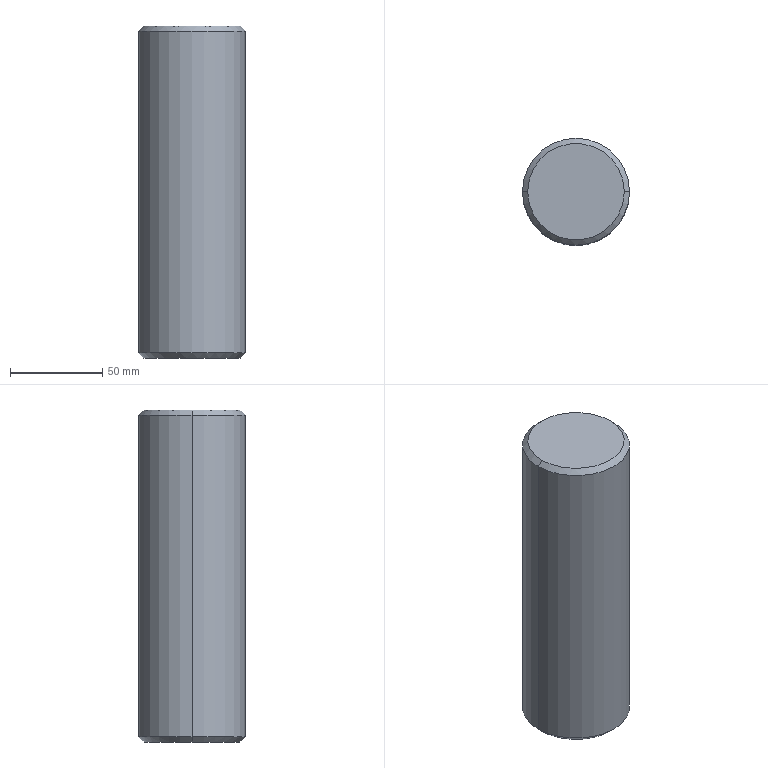Part | SolidWorks | features BaseBody 1 | 1 solid | 12 faces | box 58 x 58 x 180 mm | volume 471042 mm3 | cone 6 | cylinder 4 | plane 2 | commonest cylinder face diameters 10.5 x2 58 x2
STEP:
#1=CARTESIAN_POINT('',(74.754,163.004,-390.5));
#2=VERTEX_POINT('',#1);
#3=CARTESIAN_POINT('',(85.254,163.004,-390.5));
#4=VERTEX_POINT('',#3);
#5=CARTESIAN_POINT('',(80.004,163.004,-390.5));
#6=DIRECTION('',(0.,0.,1.));
#7=DIRECTION('',(1.,0.,0.));
#8=AXIS2_PLACEMENT_3D('',#5,#6,#7);
#9=CIRCLE('',#8,5.25);
#10=EDGE_CURVE('',#2,#4,#9,.T.);
#11=ORIENTED_EDGE('',*,*,#10,.F.);
#12=CARTESIAN_POINT('',(74.754,163.004,-355.5));
#13=VERTEX_POINT('',#12);
#14=CARTESIAN_POINT('',(74.754,163.004,-390.5));
#15=DIRECTION('',(0.,0.,1.));
#16=VECTOR('',#15,1000.);
#17=LINE('',#14,#16);
#18=EDGE_CURVE('',#2,#13,#17,.T.);
#19=ORIENTED_EDGE('',*,*,#18,.T.);
#20=CARTESIAN_POINT('',(85.254,163.004,-355.5));
#21=VERTEX_POINT('',#20);
#22=CARTESIAN_POINT('',(80.004,163.004,-355.5));
#23=DIRECTION('',(0.,0.,1.));
#24=DIRECTION('',(1.,0.,0.));
#25=AXIS2_PLACEMENT_3D('',#22,#23,#24);
#26=CIRCLE('',#25,5.25);
#27=EDGE_CURVE('',#13,#21,#26,.T.);
#28=ORIENTED_EDGE('',*,*,#27,.T.);
#29=CARTESIAN_POINT('',(85.254,163.004,-390.5));
#30=DIRECTION('',(0.,0.,1.));
#31=VECTOR('',#30,1000.);
#32=LINE('',#29,#31);
#33=EDGE_CURVE('',#4,#21,#32,.T.);
#34=ORIENTED_EDGE('',*,*,#33,.F.);
#35=EDGE_LOOP('',(#11,#19,#28,#34));
#36=FACE_OUTER_BOUND('',#35,.T.);
#37=CARTESIAN_POINT('',(80.004,163.004,-390.5));
#38=DIRECTION('',(0.,0.,1.));
#39=DIRECTION('',(1.,0.,0.));
#40=AXIS2_PLACEMENT_3D('',#37,#38,#39);
#41=CYLINDRICAL_SURFACE('',#40,5.25);
#42=ADVANCED_FACE('',(#36),#41,.F.);
#43=CARTESIAN_POINT('',(80.004,163.004,-352.345));
#44=VERTEX_POINT('',#43);
#45=CARTESIAN_POINT('',(74.754,163.004,-355.5));
#46=DIRECTION('',(-0.8572,0.,-0.515));
#47=VECTOR('',#46,1000.);
#48=LINE('',#45,#47);
#49=EDGE_CURVE('',#44,#13,#48,.T.);
#50=ORIENTED_EDGE('',*,*,#49,.F.);
#51=CARTESIAN_POINT('',(85.254,163.004,-355.5));
#52=DIRECTION('',(0.8572,0.,-0.515));
#53=VECTOR('',#52,1000.);
#54=LINE('',#51,#53);
#55=EDGE_CURVE('',#44,#21,#54,.T.);
#56=ORIENTED_EDGE('',*,*,#55,.T.);
#57=ORIENTED_EDGE('',*,*,#27,.F.);
#58=EDGE_LOOP('',(#50,#56,#57));
#59=FACE_OUTER_BOUND('',#58,.T.);
#60=CARTESIAN_POINT('',(80.004,163.004,-355.5));
#61=DIRECTION('',(0.,0.,-1.));
#62=DIRECTION('',(-1.,0.,0.));
#63=AXIS2_PLACEMENT_3D('',#60,#61,#62);
#64=CONICAL_SURFACE('',#63,5.25,1.03);
#65=ADVANCED_FACE('',(#59),#64,.F.);
#66=CARTESIAN_POINT('',(53.832,163.004,-390.5));
#67=VERTEX_POINT('',#66);
#68=CARTESIAN_POINT('',(106.175,163.004,-390.5));
#69=VERTEX_POINT('',#68);
#70=CARTESIAN_POINT('',(80.004,163.004,-390.5));
#71=DIRECTION('',(0.,0.,-1.));
#72=DIRECTION('',(1.,0.,0.));
#73=AXIS2_PLACEMENT_3D('',#70,#71,#72);
#74=CIRCLE('',#73,26.172);
#75=EDGE_CURVE('',#67,#69,#74,.T.);
#76=ORIENTED_EDGE('',*,*,#75,.F.);
#77=CARTESIAN_POINT('',(51.004,163.004,-387.672));
#78=VERTEX_POINT('',#77);
#79=CARTESIAN_POINT('',(50.418,163.004,-387.086));
#80=DIRECTION('',(-0.7071,0.,0.7071));
#81=VECTOR('',#80,1000.);
#82=LINE('',#79,#81);
#83=EDGE_CURVE('',#67,#78,#82,.T.);
#84=ORIENTED_EDGE('',*,*,#83,.T.);
#85=CARTESIAN_POINT('',(109.004,163.004,-387.672));
#86=VERTEX_POINT('',#85);
#87=CARTESIAN_POINT('',(80.004,163.004,-387.672));
#88=DIRECTION('',(0.,0.,1.));
#89=DIRECTION('',(1.,0.,0.));
#90=AXIS2_PLACEMENT_3D('',#87,#88,#89);
#91=CIRCLE('',#90,29.);
#92=EDGE_CURVE('',#86,#78,#91,.T.);
#93=ORIENTED_EDGE('',*,*,#92,.F.);
#94=CARTESIAN_POINT('',(109.589,163.004,-387.086));
#95=DIRECTION('',(0.7071,0.,0.7071));
#96=VECTOR('',#95,1000.);
#97=LINE('',#94,#96);
#98=EDGE_CURVE('',#69,#86,#97,.T.);
#99=ORIENTED_EDGE('',*,*,#98,.F.);
#100=EDGE_LOOP('',(#76,#84,#93,#99));
#101=FACE_OUTER_BOUND('',#100,.T.);
#102=CARTESIAN_POINT('',(80.004,163.004,-387.086));
#103=DIRECTION('',(0.,0.,1.));
#104=DIRECTION('',(1.,0.,0.));
#105=AXIS2_PLACEMENT_3D('',#102,#103,#104);
#106=CONICAL_SURFACE('',#105,29.586,0.7854);
#107=ADVANCED_FACE('',(#101),#106,.T.);
#108=CARTESIAN_POINT('',(106.175,163.004,-210.5));
#109=VERTEX_POINT('',#108);
#110=CARTESIAN_POINT('',(53.832,163.004,-210.5));
#111=VERTEX_POINT('',#110);
#112=CARTESIAN_POINT('',(80.004,163.004,-210.5));
#113=DIRECTION('',(0.,0.,1.));
#114=DIRECTION('',(1.,0.,0.));
#115=AXIS2_PLACEMENT_3D('',#112,#113,#114);
#116=CIRCLE('',#115,26.172);
#117=EDGE_CURVE('',#109,#111,#116,.T.);
#118=ORIENTED_EDGE('',*,*,#117,.F.);
#119=CARTESIAN_POINT('',(109.004,163.004,-213.328));
#120=VERTEX_POINT('',#119);
#121=CARTESIAN_POINT('',(107.589,163.004,-211.914));
#122=DIRECTION('',(0.7071,0.,-0.7071));
#123=VECTOR('',#122,1000.);
#124=LINE('',#121,#123);
#125=EDGE_CURVE('',#109,#120,#124,.T.);
#126=ORIENTED_EDGE('',*,*,#125,.T.);
#127=CARTESIAN_POINT('',(51.004,163.004,-213.328));
#128=VERTEX_POINT('',#127);
#129=CARTESIAN_POINT('',(80.004,163.004,-213.328));
#130=DIRECTION('',(0.,0.,-1.));
#131=DIRECTION('',(-1.,0.,0.));
#132=AXIS2_PLACEMENT_3D('',#129,#130,#131);
#133=CIRCLE('',#132,29.);
#134=EDGE_CURVE('',#128,#120,#133,.T.);
#135=ORIENTED_EDGE('',*,*,#134,.F.);
#136=CARTESIAN_POINT('',(52.418,163.004,-211.914));
#137=DIRECTION('',(-0.7071,0.,-0.7071));
#138=VECTOR('',#137,1000.);
#139=LINE('',#136,#138);
#140=EDGE_CURVE('',#111,#128,#139,.T.);
#141=ORIENTED_EDGE('',*,*,#140,.F.);
#142=EDGE_LOOP('',(#118,#126,#135,#141));
#143=FACE_OUTER_BOUND('',#142,.T.);
#144=CARTESIAN_POINT('',(80.004,163.004,-211.914));
#145=DIRECTION('',(0.,0.,-1.));
#146=DIRECTION('',(-1.,0.,0.));
#147=AXIS2_PLACEMENT_3D('',#144,#145,#146);
#148=CONICAL_SURFACE('',#147,27.586,0.7854);
#149=ADVANCED_FACE('',(#143),#148,.T.);
#150=ORIENTED_EDGE('',*,*,#134,.T.);
#151=CARTESIAN_POINT('',(109.004,163.004,-210.5));
#152=DIRECTION('',(0.,0.,-1.));
#153=VECTOR('',#152,1000.);
#154=LINE('',#151,#153);
#155=EDGE_CURVE('',#120,#86,#154,.T.);
#156=ORIENTED_EDGE('',*,*,#155,.T.);
#157=ORIENTED_EDGE('',*,*,#92,.T.);
#158=CARTESIAN_POINT('',(51.004,163.004,-210.5));
#159=DIRECTION('',(0.,0.,-1.));
#160=VECTOR('',#159,1000.);
#161=LINE('',#158,#160);
#162=EDGE_CURVE('',#128,#78,#161,.T.);
#163=ORIENTED_EDGE('',*,*,#162,.F.);
#164=EDGE_LOOP('',(#150,#156,#157,#163));
#165=FACE_OUTER_BOUND('',#164,.T.);
#166=CARTESIAN_POINT('',(80.004,163.004,-210.5));
#167=DIRECTION('',(0.,0.,-1.));
#168=DIRECTION('',(-1.,0.,0.));
#169=AXIS2_PLACEMENT_3D('',#166,#167,#168);
#170=CYLINDRICAL_SURFACE('',#169,29.);
#171=ADVANCED_FACE('',(#165),#170,.T.);
#172=ORIENTED_EDGE('',*,*,#155,.F.);
#173=CARTESIAN_POINT('',(80.004,163.004,-213.328));
#174=DIRECTION('',(0.,0.,-1.));
#175=DIRECTION('',(-1.,0.,0.));
#176=AXIS2_PLACEMENT_3D('',#173,#174,#175);
#177=CIRCLE('',#176,29.);
#178=EDGE_CURVE('',#120,#128,#177,.T.);
#179=ORIENTED_EDGE('',*,*,#178,.T.);
#180=ORIENTED_EDGE('',*,*,#162,.T.);
#181=CARTESIAN_POINT('',(80.004,163.004,-387.672));
#182=DIRECTION('',(0.,0.,1.));
#183=DIRECTION('',(1.,0.,0.));
#184=AXIS2_PLACEMENT_3D('',#181,#182,#183);
#185=CIRCLE('',#184,29.);
#186=EDGE_CURVE('',#78,#86,#185,.T.);
#187=ORIENTED_EDGE('',*,*,#186,.T.);
#188=EDGE_LOOP('',(#172,#179,#180,#187));
#189=FACE_OUTER_BOUND('',#188,.T.);
#190=CARTESIAN_POINT('',(80.004,163.004,-210.5));
#191=DIRECTION('',(0.,0.,-1.));
#192=DIRECTION('',(-1.,0.,0.));
#193=AXIS2_PLACEMENT_3D('',#190,#191,#192);
#194=CYLINDRICAL_SURFACE('',#193,29.);
#195=ADVANCED_FACE('',(#189),#194,.T.);
#196=CARTESIAN_POINT('',(80.004,163.004,-210.5));
#197=DIRECTION('',(0.,0.,1.));
#198=DIRECTION('',(1.,0.,0.));
#199=AXIS2_PLACEMENT_3D('',#196,#197,#198);
#200=CIRCLE('',#199,26.172);
#201=EDGE_CURVE('',#111,#109,#200,.T.);
#202=ORIENTED_EDGE('',*,*,#201,.T.);
#203=ORIENTED_EDGE('',*,*,#117,.T.);
#204=EDGE_LOOP('',(#202,#203));
#205=FACE_OUTER_BOUND('',#204,.T.);
#206=CARTESIAN_POINT('',(80.004,163.004,-210.5));
#207=DIRECTION('',(0.,0.,1.));
#208=DIRECTION('',(1.,0.,0.));
#209=AXIS2_PLACEMENT_3D('',#206,#207,#208);
#210=PLANE('',#209);
#211=ADVANCED_FACE('',(#205),#210,.T.);
#212=CARTESIAN_POINT('',(80.004,163.004,-390.5));
#213=DIRECTION('',(0.,0.,1.));
#214=DIRECTION('',(1.,0.,0.));
#215=AXIS2_PLACEMENT_3D('',#212,#213,#214);
#216=CIRCLE('',#215,5.25);
#217=EDGE_CURVE('',#4,#2,#216,.T.);
#218=ORIENTED_EDGE('',*,*,#217,.T.);
#219=ORIENTED_EDGE('',*,*,#10,.T.);
#220=EDGE_LOOP('',(#218,#219));
#221=FACE_BOUND('',#220,.T.);
#222=CARTESIAN_POINT('',(80.004,163.004,-390.5));
#223=DIRECTION('',(0.,0.,-1.));
#224=DIRECTION('',(1.,0.,0.));
#225=AXIS2_PLACEMENT_3D('',#222,#223,#224);
#226=CIRCLE('',#225,26.172);
#227=EDGE_CURVE('',#69,#67,#226,.T.);
#228=ORIENTED_EDGE('',*,*,#227,.T.);
#229=ORIENTED_EDGE('',*,*,#75,.T.);
#230=EDGE_LOOP('',(#228,#229));
#231=FACE_OUTER_BOUND('',#230,.T.);
#232=CARTESIAN_POINT('',(80.004,163.004,-390.5));
#233=DIRECTION('',(0.,0.,1.));
#234=DIRECTION('',(1.,0.,0.));
#235=AXIS2_PLACEMENT_3D('',#232,#233,#234);
#236=PLANE('',#235);
#237=ADVANCED_FACE('',(#221,#231),#236,.F.);
#238=ORIENTED_EDGE('',*,*,#125,.F.);
#239=ORIENTED_EDGE('',*,*,#201,.F.);
#240=ORIENTED_EDGE('',*,*,#140,.T.);
#241=ORIENTED_EDGE('',*,*,#178,.F.);
#242=EDGE_LOOP('',(#238,#239,#240,#241));
#243=FACE_OUTER_BOUND('',#242,.T.);
#244=CARTESIAN_POINT('',(80.004,163.004,-211.914));
#245=DIRECTION('',(0.,0.,-1.));
#246=DIRECTION('',(-1.,0.,0.));
#247=AXIS2_PLACEMENT_3D('',#244,#245,#246);
#248=CONICAL_SURFACE('',#247,27.586,0.7854);
#249=ADVANCED_FACE('',(#243),#248,.T.);
#250=ORIENTED_EDGE('',*,*,#83,.F.);
#251=ORIENTED_EDGE('',*,*,#227,.F.);
#252=ORIENTED_EDGE('',*,*,#98,.T.);
#253=ORIENTED_EDGE('',*,*,#186,.F.);
#254=EDGE_LOOP('',(#250,#251,#252,#253));
#255=FACE_OUTER_BOUND('',#254,.T.);
#256=CARTESIAN_POINT('',(80.004,163.004,-387.086));
#257=DIRECTION('',(0.,0.,1.));
#258=DIRECTION('',(1.,0.,0.));
#259=AXIS2_PLACEMENT_3D('',#256,#257,#258);
#260=CONICAL_SURFACE('',#259,29.586,0.7854);
#261=ADVANCED_FACE('',(#255),#260,.T.);
#262=ORIENTED_EDGE('',*,*,#55,.F.);
#263=ORIENTED_EDGE('',*,*,#49,.T.);
#264=CARTESIAN_POINT('',(80.004,163.004,-355.5));
#265=DIRECTION('',(0.,0.,1.));
#266=DIRECTION('',(1.,0.,0.));
#267=AXIS2_PLACEMENT_3D('',#264,#265,#266);
#268=CIRCLE('',#267,5.25);
#269=EDGE_CURVE('',#21,#13,#268,.T.);
#270=ORIENTED_EDGE('',*,*,#269,.F.);
#271=EDGE_LOOP('',(#262,#263,#270));
#272=FACE_OUTER_BOUND('',#271,.T.);
#273=CARTESIAN_POINT('',(80.004,163.004,-355.5));
#274=DIRECTION('',(0.,0.,-1.));
#275=DIRECTION('',(-1.,0.,0.));
#276=AXIS2_PLACEMENT_3D('',#273,#274,#275);
#277=CONICAL_SURFACE('',#276,5.25,1.03);
#278=ADVANCED_FACE('',(#272),#277,.F.);
#279=ORIENTED_EDGE('',*,*,#18,.F.);
#280=ORIENTED_EDGE('',*,*,#217,.F.);
#281=ORIENTED_EDGE('',*,*,#33,.T.);
#282=ORIENTED_EDGE('',*,*,#269,.T.);
#283=EDGE_LOOP('',(#279,#280,#281,#282));
#284=FACE_OUTER_BOUND('',#283,.T.);
#285=CARTESIAN_POINT('',(80.004,163.004,-390.5));
#286=DIRECTION('',(0.,0.,1.));
#287=DIRECTION('',(1.,0.,0.));
#288=AXIS2_PLACEMENT_3D('',#285,#286,#287);
#289=CYLINDRICAL_SURFACE('',#288,5.25);
#290=ADVANCED_FACE('',(#284),#289,.F.);
#291=CLOSED_SHELL('',(#42,#65,#107,#149,#171,#195,#211,#237,#249,#261,#278,#290));
#292=MANIFOLD_SOLID_BREP('',#291);
#293=CARTESIAN_POINT('',(0.,0.,0.));
#294=DIRECTION('',(0.,0.,1.));
#295=DIRECTION('',(1.,0.,0.));
#296=AXIS2_PLACEMENT_3D('',#293,#294,#295);
#297=(LENGTH_UNIT()NAMED_UNIT(*)SI_UNIT(.MILLI.,.METRE.));
#298=UNCERTAINTY_MEASURE_WITH_UNIT(LENGTH_MEASURE(0.00001),#297,'','');
#299=(NAMED_UNIT(*)PLANE_ANGLE_UNIT()SI_UNIT($,.RADIAN.));
#300=(NAMED_UNIT(*)SI_UNIT($,.STERADIAN.)SOLID_ANGLE_UNIT());
#301=(GEOMETRIC_REPRESENTATION_CONTEXT(3)GLOBAL_UNCERTAINTY_ASSIGNED_CONTEXT((#298))GLOBAL_UNIT_ASSIGNED_CONTEXT((#297,#299,#300))REPRESENTATION_CONTEXT('',''));
#302=ADVANCED_BREP_SHAPE_REPRESENTATION('',(#292,#296),#301);